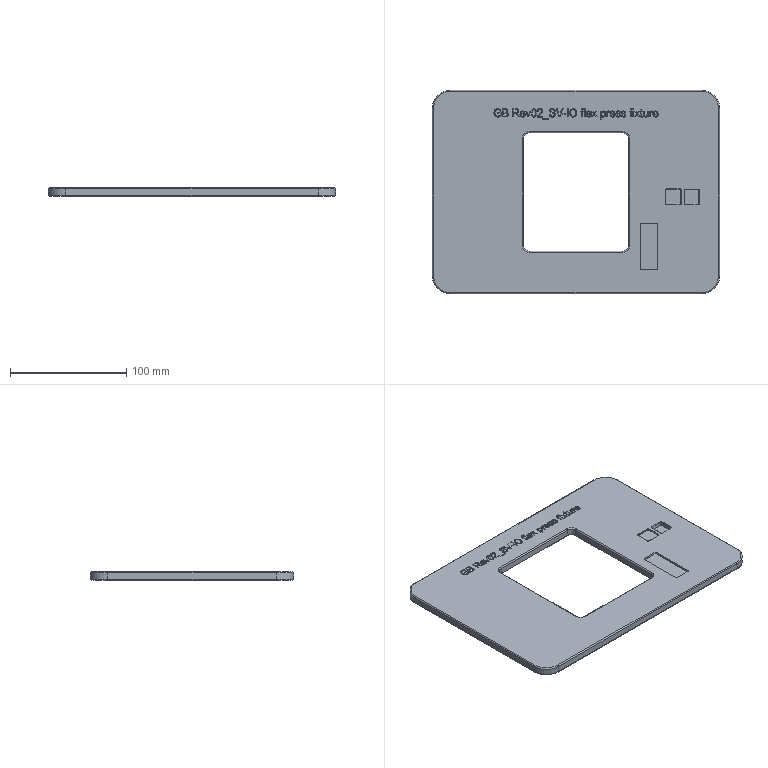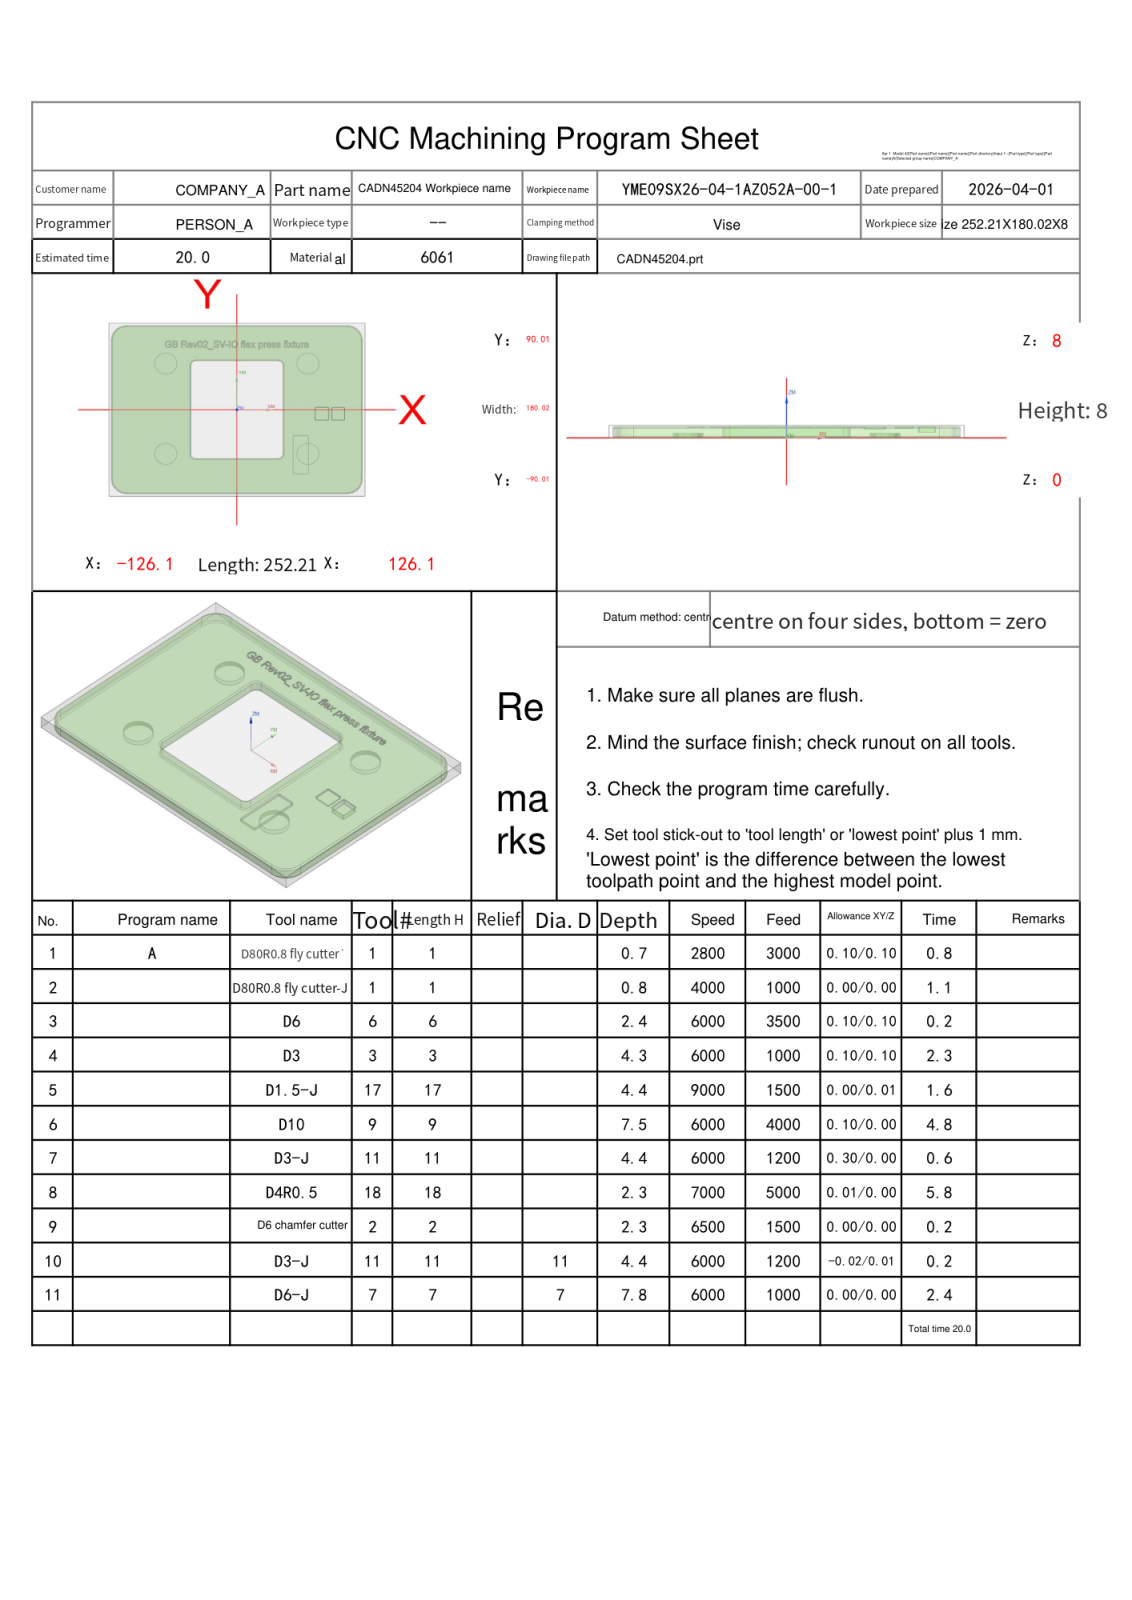NC program | NX | posted by the shop | part box 247.208 x 175.016 x 7.2 mm
Lines 7607 to 9197 of 29502:
N8 T18 M06
(D4R0.5  D=4. R=0.5 H=18 ce=0.01 di=0.00)
G00 G90 G54 X-18.349 Y50.167 M03 S7000
G43 H18 Z27.2
M08
Z8.7
G01 X-40.567 Z7.536 F5000.
X-41.143 Y50.101 Z7.505
X-41.705 Y49.958 Z7.475
X-42.242 Y49.741 Z7.444
X-42.746 Y49.455 Z7.414
X-43.207 Y49.103 Z7.384
X-43.617 Y48.693 Z7.353
X-43.968 Y48.232 Z7.323
X-44.255 Y47.729 Z7.293
X-44.472 Y47.191 Z7.262
X-44.615 Y46.629 Z7.232
X-44.681 Y46.054 Z7.201
Y45.846 Z7.191
Y-45.846
G03 X-40.359 Y-50.167 I4.322 J0.0
G01 X40.363
G03 X44.685 Y-45.846 I0.0 J4.322
G01 Y45.846
G03 X40.363 Y50.167 I-4.322 J0.0
G01 X-40.359
G03 X-44.681 Y45.846 I0.0 J-4.322
G01 X-44.682 Y43.852 Z7.19
X-44.68 Y41.859
Y39.866
X-44.679 Y37.872
Y35.879
X-44.678 Y33.886
X-44.677 Y31.893
X-44.676 Y29.899
Y27.906
X-44.675 Y25.913
X-44.674 Y23.919
X-44.673 Y21.926
X-44.672 Y19.933 Z7.189
Y17.94
X-44.671 Y15.946
X-44.67 Y13.953
X-44.669 Y11.96
Y9.966
X-44.668 Y7.973
X-44.667 Y5.98
X-44.666 Y3.987
Y1.993
X-44.665 Y0.0
X-44.664 Y-1.993
Y-3.987 Z7.188
X-44.663 Y-5.98
Y-7.973
X-44.662 Y-9.966
X-44.661 Y-11.96
X-44.66 Y-13.953
Y-15.946
X-44.659 Y-17.94
Y-19.933
X-44.658 Y-21.926
Y-23.919
X-44.656 Y-25.913 Z7.187
Y-27.906
X-44.655 Y-29.899
Y-31.893
X-44.654 Y-33.886
Y-35.879
X-44.653 Y-37.872
Y-39.866
X-44.651 Y-41.859
Y-43.852
X-44.65 Y-45.846
X-44.645 Y-46.044
X-44.632 Y-46.241
X-44.609 Y-46.438
X-44.577 Y-46.634
X-44.536 Y-46.828
X-44.486 Y-47.02
X-44.427 Y-47.209
X-44.36 Y-47.395
X-44.284 Y-47.578
X-44.2 Y-47.758
X-44.107 Y-47.933
X-44.007 Y-48.104
X-43.898 Y-48.27
X-43.783 Y-48.431
X-43.659 Y-48.586
X-43.53 Y-48.736
X-43.392 Y-48.879 Z7.186
X-43.249 Y-49.016
X-43.1 Y-49.145
X-42.944 Y-49.269
X-42.783 Y-49.384
X-42.618 Y-49.492
X-42.446 Y-49.593
X-42.271 Y-49.685
X-42.092 Y-49.769
X-41.909 Y-49.845
X-41.722 Y-49.912
X-41.533 Y-49.971
X-41.341 Y-50.02
X-41.148 Y-50.061
X-40.952 Y-50.093
X-40.755 Y-50.116
X-40.557 Y-50.129
X-40.359 Y-50.134
X-38.437
X-36.515 Y-50.133
X-34.594
X-32.672 Y-50.132
X-30.75
X-28.828 Y-50.131
X-26.906
X-24.984 Y-50.129
X-23.062 Y-50.13
X-21.14 Y-50.128
X-19.218 Z7.185
X-17.296 Y-50.127
X-15.374
X-13.452 Y-50.126
X-11.53
X-9.608 Y-50.125
X-7.686
X-5.764 Y-50.124
X-3.842
X-1.92 Y-50.122
X.002 Y-50.123
X1.924 Y-50.121
X3.846 Z7.184
X5.768 Y-50.12
X7.69
X9.612 Y-50.119
X11.534
X13.456 Y-50.118
X15.378
X17.3 Y-50.116
X19.222 Y-50.117
X21.144 Y-50.115
X23.066
X24.987 Y-50.114
X26.909 Z7.183
X28.831 Y-50.113
X30.753
X32.675 Y-50.112
X34.597
X36.519 Y-50.111
X38.441
X40.363 Y-50.11
X40.56 Y-50.105
X40.757 Y-50.092
X40.952 Y-50.069
X41.147 Y-50.037
X41.339 Y-49.996
X41.53 Y-49.947
X41.718 Y-49.889
X41.904 Y-49.822
X42.085 Y-49.746
X42.264 Y-49.662
X42.438 Y-49.57
X42.608 Y-49.471
X42.773 Y-49.363
X42.933 Y-49.248
X43.087 Y-49.126
X43.236 Y-48.996
X43.378 Y-48.86
X43.514 Y-48.718
X43.643 Y-48.569
X43.765 Y-48.415
X43.88 Y-48.255
X43.988 Y-48.09
X44.088 Y-47.92
X44.179 Y-47.746
X44.263 Y-47.567
X44.338 Y-47.386
X44.405 Y-47.2
X44.463 Y-47.012
X44.513 Y-46.822
X44.553 Y-46.629
X44.585 Y-46.434
X44.608 Y-46.239
X44.621 Y-46.042
X44.626 Y-45.846
X44.625 Y-43.852
Y-41.859 Z7.182
X44.624 Y-39.866
Y-37.872
X44.623 Y-35.879
Y-33.886
X44.622 Y-31.893
Y-29.899
X44.621 Y-27.906
Y-25.913
X44.62 Y-23.919
X44.619 Y-21.926
Y-19.933
X44.618 Y-17.94 Z7.181
Y-15.946
X44.617 Y-13.953
Y-11.96
X44.616 Y-9.966
Y-7.973
X44.615 Y-5.98
Y-3.987
X44.614 Y-1.993
Y0.0
X44.613 Y1.993
Y3.987 Z7.18
X44.612 Y5.98
Y7.973
X44.611 Y9.966
Y11.96
X44.61 Y13.953
Y15.946
X44.609 Y17.94
Y19.933
X44.608 Y21.926
Y23.919
X44.607 Y25.913
Y27.906 Z7.179
X44.606 Y29.899
Y31.893
X44.605 Y33.886
Y35.879
X44.604 Y37.872
Y39.866
X44.602 Y41.859
X44.603 Y43.852
X44.601 Y45.846
X44.597 Y46.041
X44.583 Y46.237
X44.561 Y46.431
X44.529 Y46.624
X44.489 Y46.816
X44.439 Y47.005
X44.381 Y47.192
X44.315 Y47.376
X44.24 Y47.557
X44.157 Y47.734
X44.065 Y47.908
X43.966 Y48.076
X43.859 Y48.24
X43.745 Y48.399
X43.623 Y48.553
X43.495 Y48.7
X43.36 Y48.842
X43.218 Y48.977
X43.07 Y49.106
X42.917 Y49.227
X42.758 Y49.341
X42.594 Y49.448
X42.425 Y49.547
X42.252 Y49.638 Z7.178
X42.075 Y49.722
X41.894 Y49.796
X41.71 Y49.863
X41.523 Y49.921
X41.333 Y49.97
X41.142 Y50.01
X40.949 Y50.042
X40.754 Y50.064
X40.559 Y50.078
X40.363 Y50.082
X38.441 Y50.083
X36.519 Y50.081
X34.597 Y50.082
X32.675 Y50.08
X30.753 Y50.081
X28.831 Y50.079
X26.909 Y50.08
X24.987 Y50.078
X23.066 Y50.079
X21.144 Y50.078
X19.222
X17.3 Y50.077 Z7.177
X15.378
X13.456 Y50.076
X11.534
X9.612 Y50.075
X7.69
X5.768 Y50.074
X3.846
X1.924 Y50.073
X.002
X-1.92 Y50.072
X-3.842
X-5.764 Y50.071 Z7.176
X-7.686
X-9.608 Y50.07
X-11.53
X-13.452 Y50.069
X-15.374
X-17.296
X-19.218 Y50.068
X-21.14
X-23.062 Y50.067
X-24.984
X-26.906 Y50.066
X-28.828 Z7.175
X-30.75 Y50.065
X-32.672
X-34.594 Y50.064
X-36.515
X-38.437
X-40.359 Y50.063
X-40.554 Y50.058
X-40.749 Y50.045
X-40.942 Y50.022
X-41.134 Y49.991
X-41.325 Y49.951
X-41.514 Y49.902
X-41.7 Y49.844
X-41.883 Y49.778
X-42.063 Y49.703
X-42.239 Y49.621
X-42.411 Y49.529
X-42.579 Y49.431
X-42.742 Y49.324
X-42.901 Y49.211
X-43.053 Y49.09
X-43.2 Y48.962
X-43.341 Y48.827
X-43.476 Y48.686
X-43.603 Y48.539
X-43.724 Y48.387
X-43.838 Y48.228
X-43.944 Y48.065
X-44.043 Y47.897
X-44.134 Y47.725
X-44.216 Y47.549
X-44.291 Y47.369
X-44.357 Y47.185
X-44.415 Y46.999
X-44.463 Y46.811
X-44.504 Y46.62
X-44.535 Y46.428
X-44.558 Y46.235
X-44.571 Y46.04
X-44.575 Y45.846
Y43.852
X-44.574 Y41.859 Z7.174
X-44.573 Y39.866
Y37.872
X-44.572 Y35.879
Y33.886
X-44.571 Y31.893
X-44.57 Y29.899
X-44.569 Y27.906
Y25.913 Z7.173
X-44.568 Y23.919
Y21.926
X-44.567 Y19.933
X-44.566 Y17.94
Y15.946
X-44.565 Y13.953
Y11.96
X-44.564 Y9.966
Y7.973 Z7.172
X-44.563 Y5.98
X-44.562 Y3.987
X-44.561 Y1.993
Y0.0
X-44.56 Y-1.993
Y-3.987
X-44.559 Y-5.98
Y-7.973 Z7.171
X-44.558 Y-9.966
Y-11.96
X-44.556 Y-13.953
X-44.557 Y-15.946
X-44.555 Y-17.94
Y-19.933
X-44.554 Y-21.926
Y-23.919 Z7.17
X-44.553 Y-25.913
Y-27.906
X-44.552 Y-29.899
Y-31.893
X-44.55 Y-33.886
X-44.551 Y-35.879
X-44.549 Y-37.872
Y-39.866 Z7.169
X-44.548 Y-41.859
Y-43.852
X-44.547 Y-45.846
X-44.542 Y-46.039
X-44.529 Y-46.232
X-44.507 Y-46.424
X-44.476 Y-46.615
X-44.435 Y-46.804
X-44.387 Y-46.991
X-44.329 Y-47.176
X-44.264 Y-47.358
X-44.19 Y-47.537
X-44.108 Y-47.712
X-44.017 Y-47.883
X-43.919 Y-48.05
X-43.813 Y-48.212
X-43.701 Y-48.369
X-43.58 Y-48.52
X-43.453 Y-48.666
X-43.32 Y-48.806
X-43.18 Y-48.94
X-43.034 Y-49.066
X-42.882 Y-49.186
X-42.725 Y-49.299
X-42.563 Y-49.405
X-42.396 Y-49.503
X-42.225 Y-49.593
X-42.05 Y-49.675
X-41.872 Y-49.749
X-41.69 Y-49.814
X-41.505 Y-49.872
X-41.318 Y-49.92
X-41.129 Y-49.96
X-40.938 Y-49.991
X-40.746 Y-50.014
X-40.553 Y-50.027
X-40.359 Y-50.031
X-38.437
X-36.515 Y-50.03
X-34.594 Z7.168
X-32.672 Y-50.029
X-30.75
X-28.828 Y-50.028
X-26.906
X-24.984 Y-50.027
X-23.062
X-21.14 Y-50.026
X-19.218 Z7.167
X-17.296 Y-50.025
X-15.374 Y-50.024
X-13.452
X-11.53 Y-50.023
X-9.608 Y-50.022
X-7.686
X-5.764 Y-50.021
X-3.842
X-1.92 Y-50.02 Z7.166
X.002
X1.924 Y-50.019
X3.846
X5.768 Y-50.018
X7.69
X9.612 Y-50.017
X11.534
X13.456 Y-50.016 Z7.165
X15.378 Y-50.015
X17.3
X19.222 Y-50.014
X21.144
X23.066 Y-50.013
X24.987
X26.909 Y-50.012
X28.831 Y-50.011
X30.753 Z7.164
X32.675 Y-50.01
X34.597
X36.519 Y-50.009
X38.441
X40.363 Y-50.008
X40.555 Y-50.004
X40.747 Y-49.991
X40.938 Y-49.969
X41.128 Y-49.937
X41.316 Y-49.898
X41.502 Y-49.849
X41.686 Y-49.792
X41.867 Y-49.727
X42.045 Y-49.653
X42.219 Y-49.571
X42.389 Y-49.482
X42.554 Y-49.384
X42.716 Y-49.279
X42.871 Y-49.167
X43.022 Y-49.048
X43.167 Y-48.921
X43.306 Y-48.789
X43.439 Y-48.649
X43.565 Y-48.504
X43.684 Y-48.354
X43.797 Y-48.198
X43.902 Y-48.036
X43.999 Y-47.871
X44.089 Y-47.701
X44.17 Y-47.527
X44.244 Y-47.349
X44.309 Y-47.168
X44.366 Y-46.984
X44.414 Y-46.798
X44.454 Y-46.61
X44.485 Y-46.42 Z7.163
X44.507 Y-46.23
X44.52 Y-46.038
X44.524 Y-45.846
Y-43.852
X44.523 Y-41.859
Y-39.866
X44.522 Y-37.872
Y-35.879
X44.521 Y-33.886
Y-31.893
X44.52 Y-29.899 Z7.162
Y-27.906
X44.519 Y-25.913
Y-23.919
X44.518 Y-21.926
Y-19.933
X44.517 Y-17.94
Y-15.946
X44.516 Y-13.953
Y-11.96 Z7.161
X44.515 Y-9.966
Y-7.973
X44.514 Y-5.98
Y-3.987
X44.513 Y-1.993
Y0.0
X44.512 Y1.993
Y3.987 Z7.16
X44.511 Y5.98
Y7.973
X44.51 Y9.966
Y11.96
X44.509 Y13.953
Y15.946
X44.508 Y17.94
Y19.933 Z7.159
X44.507 Y21.926
Y23.919
X44.506 Y25.913
Y27.906
X44.505 Y29.899
Y31.893
X44.504 Y33.886
Y35.879
X44.503 Y37.872 Z7.158
Y39.866
X44.502 Y41.859
Y43.852
X44.501 Y45.846
X44.496 Y46.037
X44.483 Y46.227
X44.461 Y46.417
X44.43 Y46.606
X44.391 Y46.793
X44.342 Y46.978
X44.286 Y47.16
X44.221 Y47.34
X44.148 Y47.517
X44.066 Y47.689
X43.977 Y47.859
X43.88 Y48.023
X43.776 Y48.183
X43.664 Y48.338
X43.546 Y48.488
X43.42 Y48.632
X43.288 Y48.771
X43.15 Y48.902
X43.006 Y49.028
X42.856 Y49.146
X42.701 Y49.258
X42.541 Y49.362
X42.376 Y49.459
X42.207 Y49.548
X42.034 Y49.629
X41.857 Y49.702
X41.678 Y49.767
X41.495 Y49.824
X41.31 Y49.872
X41.123 Y49.911
X40.935 Y49.942
X40.745 Y49.964
X40.554 Y49.977
X40.363 Y49.981
X38.441 Z7.157
X36.519 Y49.98
X34.597
X32.675 Y49.979
X30.753
X28.831 Y49.978
X26.909
X24.987 Y49.977
X23.066 Z7.156
X21.144 Y49.976
X19.222
X17.3
X15.378
X13.456 Y49.975
X11.534
X9.612 Y49.974
X7.69
X5.768 Y49.973 Z7.155
X3.846
X1.924 Y49.972
X.002
X-1.92 Y49.971
X-3.842
X-5.764 Y49.97
X-7.686
X-9.608 Y49.969 Z7.154
X-11.53
X-13.452 Y49.968
X-15.374
X-17.296 Y49.967
X-19.218
X-21.14 Y49.966
X-23.062
X-24.984
X-26.906 Y49.965 Z7.153
X-28.828
X-30.75 Y49.964
X-32.672
X-34.594 Y49.963
X-36.515
X-38.437 Y49.962
X-40.359
X-40.55 Y49.957
X-40.739 Y49.944
X-40.928 Y49.922
X-41.116 Y49.892
X-41.302 Y49.852
X-41.486 Y49.805
X-41.667 Y49.748
X-41.846 Y49.684
X-42.022 Y49.611
X-42.194 Y49.53
X-42.362 Y49.441
X-42.526 Y49.345 Z7.152
X-42.685 Y49.241
X-42.84 Y49.13
X-42.989 Y49.012
X-43.132 Y48.887
X-43.27 Y48.756
X-43.401 Y48.618
X-43.526 Y48.475
X-43.644 Y48.326
X-43.755 Y48.171
X-43.858 Y48.012
X-43.955 Y47.848
X-44.043 Y47.68
X-44.124 Y47.508
X-44.197 Y47.332
X-44.261 Y47.153
X-44.317 Y46.972
X-44.365 Y46.788
X-44.404 Y46.602
X-44.435 Y46.414
X-44.457 Y46.225
X-44.47 Y46.036
X-44.474 Y45.846
Y43.852
X-44.473 Y41.859
X-44.472 Y39.866
Y37.872
X-44.471 Y35.879 Z7.151
Y33.886
X-44.47 Y31.893
X-44.469 Y29.899
Y27.906
X-44.468 Y25.913
Y23.919
X-44.467 Y21.926 Z7.15
Y19.933
X-44.466 Y17.94
Y15.946
X-44.465 Y13.953
Y11.96
X-44.464 Y9.966 Z7.149
X-44.463 Y7.973
X-44.462 Y5.98
Y3.987
X-44.461 Y1.993
Y0.0
X-44.46 Y-1.993
Y-3.987 Z7.148
X-44.459 Y-5.98
Y-7.973
X-44.458 Y-9.966
Y-11.96
X-44.456 Y-13.953
X-44.457 Y-15.946 Z7.147
X-44.455 Y-17.94
Y-19.933
X-44.454 Y-21.926
Y-23.919
X-44.453 Y-25.913
Y-27.906 Z7.146
X-44.452 Y-29.899
Y-31.893
X-44.451 Y-33.886
Y-35.879
X-44.45 Y-37.872
Y-39.866
X-44.449 Y-41.859 Z7.145
Y-43.852
X-44.448 Y-45.846
X-44.442 Y-46.046
X-44.428 Y-46.246
X-44.403 Y-46.445
X-44.369 Y-46.643
X-44.325 Y-46.839
X-44.271 Y-47.032
X-44.208 Y-47.223
X-44.136 Y-47.41
X-44.054 Y-47.593
X-43.964 Y-47.772
X-43.865 Y-47.947
X-43.758 Y-48.116
X-43.642 Y-48.28
X-43.519 Y-48.439
X-43.388 Y-48.59
X-43.25 Y-48.736
X-43.104 Y-48.874
X-42.952 Y-49.005
X-42.794 Y-49.128
X-42.63 Y-49.244
X-42.46 Y-49.351
X-42.286 Y-49.45
X-42.107 Y-49.54
X-41.923 Y-49.621
X-41.736 Y-49.693
X-41.546 Y-49.756
X-41.352 Y-49.81
X-41.157 Y-49.854
X-40.959 Y-49.888
X-40.76 Y-49.912
X-40.56 Y-49.927
X-40.359 Y-49.932
X-38.437 Z7.144
X-36.515 Y-49.931
X-34.594
X-32.672 Y-49.93
X-30.75
X-28.828 Y-49.929
X-26.906 Y-49.928
X-24.984 Z7.143
X-23.062 Y-49.927
X-21.14
X-19.218 Y-49.926
X-17.296
X-15.374 Y-49.925
X-13.452 Z7.142
X-11.53 Y-49.924
X-9.608 Y-49.923
X-7.686
X-5.764 Y-49.922
X-3.842
X-1.92 Y-49.921
X.002 Z7.141
X1.924 Y-49.92
X3.846
X5.768 Y-49.919
X7.69
X9.612 Y-49.918
X11.534 Y-49.917
X13.456 Z7.14
X15.378 Y-49.916
X17.3
X19.222
X21.144 Y-49.915
X23.066
X24.987 Y-49.914
X26.909 Z7.139
X28.831 Y-49.913
X30.753
X32.675 Y-49.912
X34.597
X36.519 Y-49.911
X38.441 Z7.138
X40.363 Y-49.91
X40.563 Y-49.905
X40.762 Y-49.89
X40.96 Y-49.866
X41.156 Y-49.832
X41.351 Y-49.788
X41.543 Y-49.735
X41.732 Y-49.672
X41.918 Y-49.6
X42.101 Y-49.519
X42.279 Y-49.429
X42.452 Y-49.331
X42.621 Y-49.224
X42.784 Y-49.11
X42.941 Y-48.987
X43.092 Y-48.856
X43.237 Y-48.719
X43.374 Y-48.574
X43.504 Y-48.423
X43.627 Y-48.266
X43.742 Y-48.103
X43.848 Y-47.934
X43.947 Y-47.761
X44.036 Y-47.583
X44.117 Y-47.4
X44.189 Y-47.214
X44.251 Y-47.025
X44.304 Y-46.833
X44.348 Y-46.638
X44.382 Y-46.442
X44.406 Y-46.244
X44.421 Y-46.045
X44.426 Y-45.846
Y-43.852
X44.425 Y-41.859 Z7.137
Y-39.866
X44.424 Y-37.872
Y-35.879
X44.423 Y-33.886
Y-31.893
X44.422 Y-29.899
Y-27.906 Z7.136
X44.421 Y-25.913
Y-23.919
X44.42 Y-21.926
Y-19.933
X44.419 Y-17.94
Y-15.946 Z7.135
X44.418 Y-13.953
Y-11.96
X44.417 Y-9.966
Y-7.973
X44.416 Y-5.98
Y-3.987
X44.415 Y-1.993 Z7.134
Y0.0
X44.414 Y1.993
Y3.987
X44.413 Y5.98
Y7.973
X44.412 Y9.966 Z7.133
Y11.96
X44.411 Y13.953
Y15.946
X44.41 Y17.94
Y19.933
X44.409 Y21.926
Y23.919 Z7.132
X44.408 Y25.913
Y27.906
X44.407 Y29.899
Y31.893
X44.406 Y33.886
Y35.879 Z7.131
X44.405 Y37.872
Y39.866
X44.404 Y41.859
Y43.852
X44.403 Y45.846
X44.398 Y46.044
X44.383 Y46.241
X44.359 Y46.438
X44.325 Y46.634
X44.281 Y46.827
X44.228 Y47.018
X44.166 Y47.206
X44.095 Y47.391
X44.014 Y47.572
X43.925 Y47.749
X43.827 Y47.922 Z7.13
X43.721 Y48.089
X43.607 Y48.251
X43.485 Y48.408
X43.356 Y48.558
X43.219 Y48.701
X43.075 Y48.838
X42.925 Y48.967
X42.769 Y49.089
X42.607 Y49.203
X42.439 Y49.309
X42.267 Y49.407
X42.09 Y49.496
X41.909 Y49.576
X41.724 Y49.648
X41.535 Y49.71
X41.344 Y49.763
X41.151 Y49.806
X40.956 Y49.84
X40.759 Y49.864
X40.561 Y49.879
X40.363 Y49.883
X38.441
X36.519 Y49.882
X34.597
X32.675 Y49.881
X30.753 Y49.882 Z7.129
X28.831 Y49.88
X26.909 Y49.881
X24.987 Y49.879
X23.066 Y49.88
X21.144 Y49.879
X19.222
X17.3 Y49.878 Z7.128
X15.378
X13.456 Y49.877
X11.534
X9.612 Y49.876
X7.69
X5.768 Y49.875 Z7.127
X3.846
X1.924 Y49.874
X.002
X-1.92 Y49.873
X-3.842
X-5.764 Y49.872
X-7.686 Z7.126
X-9.608 Y49.871
X-11.53
X-13.452 Y49.87
X-15.374
X-17.296
X-19.218 Y49.869
X-21.14 Z7.125
X-23.062 Y49.868
X-24.984
X-26.906 Y49.867
X-28.828
X-30.75
X-32.672 Y49.866 Z7.124
X-34.594
X-36.515 Y49.865
X-38.437
X-40.359 Y49.864
X-40.557 Y49.859
X-40.753 Y49.845
X-40.949 Y49.82
X-41.143 Y49.787
X-41.336 Y49.743
X-41.526 Y49.691
X-41.713 Y49.629
X-41.897 Y49.558
X-42.077 Y49.478
X-42.254 Y49.389
X-42.425 Y49.292
X-42.592 Y49.186
X-42.753 Y49.073
X-42.908 Y48.951
X-43.058 Y48.822
X-43.2 Y48.687
X-43.336 Y48.544
X-43.465 Y48.394
X-43.586 Y48.239
X-43.7 Y48.078
X-43.805 Y47.911
X-43.903 Y47.739
X-43.991 Y47.563
X-44.071 Y47.383
X-44.142 Y47.199 Z7.123
X-44.204 Y47.012
X-44.256 Y46.822
X-44.299 Y46.629
X-44.333 Y46.435
X-44.357 Y46.239
X-44.371 Y46.043
X-44.376 Y45.846
Y43.852
X-44.375 Y41.859
Y39.866
X-44.374 Y37.872
Y35.879 Z7.122
X-44.373 Y33.886
Y31.893
X-44.372 Y29.899
Y27.906
X-44.371 Y25.913 Z7.121
X-44.37 Y23.919
Y21.926
X-44.369 Y19.933
X-44.368 Y17.94
Y15.946
X-44.367 Y13.953 Z7.12
Y11.96
X-44.366 Y9.966
Y7.973
X-44.365 Y5.98
Y3.987 Z7.119
X-44.364 Y1.993
Y0.0
X-44.363 Y-1.993
Y-3.987
X-44.362 Y-5.98 Z7.118
Y-7.973
X-44.361 Y-9.966
Y-11.96
X-44.359 Y-13.953
Y-15.946
X-44.358 Y-17.94 Z7.117
Y-19.933
X-44.357 Y-21.926
Y-23.919
X-44.356 Y-25.913
Y-27.906 Z7.116
X-44.355 Y-29.899
Y-31.893
X-44.354 Y-33.886
Y-35.879
X-44.353 Y-37.872 Z7.115
Y-39.866
X-44.352 Y-41.859
Y-43.852
X-44.351 Y-45.846
X-44.346 Y-46.041
X-44.332 Y-46.237
X-44.307 Y-46.431
X-44.274 Y-46.624
X-44.231 Y-46.815
X-44.179 Y-47.004
X-44.117 Y-47.19
X-44.047 Y-47.373
X-43.967 Y-47.552 Z7.114
X-43.879 Y-47.727
X-43.782 Y-47.897
X-43.678 Y-48.063
X-43.565 Y-48.223
X-43.444 Y-48.377
X-43.316 Y-48.525
X-43.181 Y-48.667
X-43.039 Y-48.802
X-42.891 Y-48.93
X-42.736 Y-49.051
X-42.576 Y-49.163
X-42.411 Y-49.268
X-42.24 Y-49.365
X-42.065 Y-49.453
X-41.886 Y-49.532
X-41.704 Y-49.602
X-41.518 Y-49.664
X-41.329 Y-49.716
X-41.138 Y-49.759
X-40.945 Y-49.792
X-40.751 Y-49.816
X-40.555 Y-49.83
X-40.359 Y-49.835
X-38.437
X-36.515 Y-49.834
X-34.594
X-32.672 Y-49.833 Z7.113
X-30.75
X-28.828 Y-49.832
X-26.906
X-24.984 Y-49.831
X-23.062 Z7.112
X-21.14 Y-49.83
X-19.218
X-17.296 Y-49.829
X-15.374
X-13.452 Y-49.828
X-11.53 Z7.111
X-9.608 Y-49.827
X-7.686
X-5.764 Y-49.826
X-3.842
X-1.92 Y-49.825 Z7.11
X.002
X1.924 Y-49.824
X3.846
X5.768 Y-49.823
X7.69 Z7.109
X9.612 Y-49.822
X11.534
X13.456 Y-49.821
X15.378
X17.3 Y-49.82
X19.222 Z7.108
X21.144 Y-49.819
X23.066
X24.987 Y-49.818
X26.909
X28.831 Y-49.817 Z7.107
X30.753
X32.675 Y-49.816
X34.597
X36.519 Y-49.815
X38.441
X40.363 Y-49.814 Z7.106
X40.558 Y-49.809
X40.752 Y-49.795
X40.945 Y-49.771
X41.137 Y-49.738
X41.327 Y-49.695
X41.515 Y-49.643
X41.7 Y-49.582
X41.882 Y-49.512
X42.06 Y-49.433
X42.234 Y-49.345
X42.403 Y-49.249
X42.568 Y-49.145
X42.727 Y-49.033
X42.88 Y-48.913
X43.028 Y-48.785
X43.169 Y-48.651
X43.303 Y-48.51
X43.43 Y-48.363
X43.55 Y-48.209
X43.662 Y-48.05
X43.766 Y-47.885
X43.862 Y-47.716
X43.95 Y-47.542
X44.028 Y-47.364
X44.099 Y-47.182
X44.16 Y-46.997
X44.211 Y-46.81
X44.254 Y-46.619
X44.287 Y-46.428
X44.311 Y-46.234
X44.325 Y-46.04
X44.33 Y-45.846
Y-43.852
X44.329 Y-41.859 Z7.105
Y-39.866
X44.328 Y-37.872
Y-35.879
X44.327 Y-33.886
Y-31.893 Z7.104
X44.326 Y-29.899
Y-27.906
X44.325 Y-25.913
Y-23.919
X44.324 Y-21.926
Y-19.933 Z7.103
X44.323 Y-17.94
Y-15.946
X44.322 Y-13.953
Y-11.96
X44.321 Y-9.966 Z7.102
Y-7.973
X44.32 Y-5.98
Y-3.987
X44.319 Y-1.993
Y0.0 Z7.101
X44.318 Y1.993
Y3.987
X44.317 Y5.98
Y7.973
X44.316 Y9.966 Z7.1
Y11.96
X44.315 Y13.953
Y15.946
X44.314 Y17.94
Y19.933
X44.313 Y21.926 Z7.099
Y23.919
X44.312 Y25.913
Y27.906
X44.311 Y29.899
Y31.893 Z7.098
X44.31 Y33.886
Y35.879
X44.309 Y37.872
Y39.866
X44.308 Y41.859 Z7.097
Y43.852
X44.307 Y45.846
X44.302 Y46.039
X44.288 Y46.232
X44.264 Y46.424
X44.231 Y46.615
X44.189 Y46.804
X44.137 Y46.99
X44.076 Y47.174
X44.007 Y47.355
X43.928 Y47.532
X43.841 Y47.705
X43.746 Y47.873
X43.642 Y48.036
X43.531 Y48.195
X43.412 Y48.347
X43.285 Y48.494
X43.152 Y48.634
X43.011 Y48.767
X42.865 Y48.894
X42.712 Y49.013
X42.554 Y49.124
X42.39 Y49.228
X42.222 Y49.323
X42.049 Y49.41
X41.872 Y49.488
X41.692 Y49.558
X41.508 Y49.619
X41.321 Y49.67
X41.132 Y49.713
X40.942 Y49.746
X40.75 Y49.769
X40.557 Y49.783 Z7.096
X40.363 Y49.788
X38.441
X36.519 Y49.787
X34.597
X32.675 Y49.786
X30.753
X28.831 Y49.785 Z7.095
X26.909
X24.987 Y49.784
X23.066
X21.144 Y49.783
X19.222 Z7.094
X17.3 Y49.782
X15.378
X13.456
X11.534 Y49.781
X9.612
X7.69 Y49.78 Z7.093
X5.768
X3.846 Y49.779
X1.924
X.002 Y49.778
X-1.92 Z7.092
X-3.842 Y49.777
X-5.764
X-7.686
X-9.608 Y49.776
X-11.53
X-13.452 Y49.775 Z7.091
X-15.374
X-17.296 Y49.774
X-19.218
X-21.14
X-23.062 Y49.773 Z7.09
X-24.984
X-26.906 Y49.772
X-28.828
X-30.75 Y49.771
X-32.672
X-34.594 Y49.77 Z7.089
X-36.515
X-38.437 Y49.769
X-40.359
X-40.552 Y49.764
X-40.744 Y49.75
X-40.935 Y49.726
X-41.125 Y49.693
X-41.313 Y49.651
X-41.498 Y49.6
X-41.681 Y49.539
X-41.861 Y49.47
X-42.037 Y49.392
X-42.209 Y49.305
X-42.376 Y49.21
X-42.539 Y49.107
X-42.696 Y48.996
X-42.848 Y48.878
X-42.994 Y48.752
X-43.133 Y48.619
X-43.266 Y48.48 Z7.088
X-43.392 Y48.334
X-43.51 Y48.182
X-43.621 Y48.025
X-43.724 Y47.862
X-43.819 Y47.695
X-43.905 Y47.523
X-43.983 Y47.347
X-44.052 Y47.167
X-44.113 Y46.984
X-44.164 Y46.799
X-44.206 Y46.611
X-44.239 Y46.421
X-44.263 Y46.23
X-44.277 Y46.038
X-44.281 Y45.846
Y43.852
X-44.28 Y41.859
Y39.866
X-44.279 Y37.872 Z7.087
Y35.879
X-44.278 Y33.886
Y31.893
X-44.277 Y29.899 Z7.086
Y27.906
X-44.276 Y25.913
Y23.919
X-44.275 Y21.926
Y19.933 Z7.085
X-44.274 Y17.94
X-44.273 Y15.946
Y13.953
X-44.272 Y11.96 Z7.084
Y9.966
X-44.271 Y7.973
Y5.98
X-44.27 Y3.987
X-44.269 Y1.993 Z7.083
Y0.0
X-44.268 Y-1.993
Y-3.987
X-44.267 Y-5.98 Z7.082
Y-7.973
X-44.266 Y-9.966
Y-11.96
X-44.265 Y-13.953
Y-15.946 Z7.081
X-44.264 Y-17.94
Y-19.933
X-44.263 Y-21.926
Y-23.919 Z7.08
X-44.262 Y-25.913
X-44.261 Y-27.906
Y-29.899
X-44.26 Y-31.893
Y-33.886 Z7.079
X-44.259 Y-35.879
Y-37.872
X-44.258 Y-39.866
Y-41.859 Z7.078
X-44.257 Y-43.852
Y-45.846
X-44.252 Y-46.037
X-44.238 Y-46.228
X-44.215 Y-46.417
X-44.182 Y-46.606
X-44.14 Y-46.793
X-44.089 Y-46.977
X-44.029 Y-47.158
X-43.96 Y-47.337
X-43.882 Y-47.512
X-43.796 Y-47.683
X-43.702 Y-47.849
X-43.6 Y-48.011
X-43.489 Y-48.167
X-43.372 Y-48.318
X-43.247 Y-48.462
X-43.115 Y-48.601
X-42.976 Y-48.733
X-42.831 Y-48.858
X-42.681 Y-48.975
X-42.524 Y-49.085
X-42.363 Y-49.188 Z7.077
X-42.196 Y-49.282
X-42.025 Y-49.368
X-41.85 Y-49.445
X-41.672 Y-49.514
X-41.49 Y-49.574
X-41.306 Y-49.625
X-41.12 Y-49.667
X-40.931 Y-49.699
X-40.741 Y-49.723
X-40.551 Y-49.737
X-40.359 Y-49.742
X-38.437 Y-49.741
X-36.515
X-34.594 Y-49.74
X-32.672 Z7.076
X-30.75 Y-49.739
X-28.828
X-26.906 Y-49.738
X-24.984
X-23.062 Y-49.737 Z7.075
X-21.14
X-19.218 Y-49.736
X-17.296
X-15.374 Y-49.735 Z7.074
X-13.452
X-11.53 Y-49.734
X-9.608
X-7.686 Y-49.733
X-5.764 Z7.073
X-3.842 Y-49.732
X-1.92
X.002 Y-49.731
X1.924
X3.846 Y-49.73 Z7.072
X5.768
X7.69 Y-49.729
X9.612
X11.534 Y-49.728 Z7.071
X13.456
X15.378 Y-49.727
X17.3
X19.222 Y-49.726
X21.144 Z7.07
X23.066 Y-49.725
X24.987
X26.909 Y-49.724
X28.831
X30.753 Y-49.723 Z7.069
X32.675
X34.597 Y-49.722
X36.519
X38.441 Y-49.721 Z7.068
X40.363
X40.553 Y-49.716
X40.743 Y-49.702
X40.932 Y-49.679
X41.119 Y-49.646
X41.305 Y-49.605
X41.488 Y-49.554
X41.669 Y-49.494
X41.846 Y-49.425
X42.02 Y-49.349
X42.19 Y-49.263
X42.355 Y-49.169
X42.516 Y-49.067
X42.671 Y-48.958
X42.821 Y-48.841
X42.965 Y-48.717
X43.103 Y-48.585
X43.234 Y-48.448
X43.358 Y-48.303
X43.475 Y-48.154
X43.585 Y-47.998
X43.686 Y-47.837
X43.78 Y-47.672
X43.866 Y-47.502
X43.942 Y-47.328
X44.011 Y-47.151
X44.07 Y-46.97
X44.121 Y-46.787
X44.163 Y-46.601
X44.195 Y-46.414
X44.218 Y-46.225
X44.232 Y-46.036
X44.237 Y-45.846
Y-43.852 Z7.067
X44.236 Y-41.859
Y-39.866
X44.235 Y-37.872
Y-35.879 Z7.066
X44.234 Y-33.886
Y-31.893
X44.233 Y-29.899
Y-27.906
X44.232 Y-25.913 Z7.065
Y-23.919
X44.231 Y-21.926
Y-19.933
X44.23 Y-17.94 Z7.064
Y-15.946
X44.229 Y-13.953
Y-11.96
X44.228 Y-9.966
Y-7.973 Z7.063
X44.227 Y-5.98
Y-3.987
X44.226 Y-1.993
Y0.0 Z7.062
X44.225 Y1.993
Y3.987
X44.224 Y5.98
Y7.973
X44.223 Y9.966 Z7.061
Y11.96
X44.222 Y13.953
Y15.946
Y17.94 Z7.06
X44.221 Y19.933
Y21.926
X44.22 Y23.919
Y25.913
X44.219 Y27.906 Z7.059
Y29.899
X44.218 Y31.893
Y33.886
X44.217 Y35.879 Z7.058
Y37.872
X44.216 Y39.866
Y41.859
X44.215 Y43.852 Z7.057
Y45.846
X44.21 Y46.035
X44.196 Y46.223
X44.173 Y46.411
X44.141 Y46.597
X44.099 Y46.781
X44.049 Y46.964
X43.989 Y47.143
X43.921 Y47.319
X43.845 Y47.492
X43.76 Y47.661
X43.666 Y47.825
X43.565 Y47.985
X43.456 Y48.14
X43.34 Y48.289
X43.217 Y48.432
X43.086 Y48.569
X42.949 Y48.699
X42.806 Y48.822
X42.657 Y48.939
X42.503 Y49.047
X42.343 Y49.148
X42.178 Y49.241
X42.01 Y49.326
X41.837 Y49.403
X41.66 Y49.471
X41.481 Y49.53
X41.299 Y49.581
X41.114 Y49.622
X40.928 Y49.654
X40.741 Y49.677
X40.552 Y49.691
X40.363 Y49.696
X38.441 Y49.695 Z7.056
X36.519
X34.597
X32.675 Y49.694
X30.753
X28.831 Y49.693 Z7.055
X26.909
X24.987 Y49.692
X23.066
X21.144 Y49.691 Z7.054
X19.222
X17.3 Y49.69
X15.378
X13.456 Y49.689
X11.534 Z7.053
X9.612 Y49.688
X7.69
X5.768 Y49.687
X3.846
X1.924 Z7.052
X.002 Y49.686
X-1.92
X-3.842
X-5.764 Y49.685 Z7.051
X-7.686
X-9.608 Y49.684
X-11.53
X-13.452 Y49.683
X-15.374 Z7.05
X-17.296 Y49.682
X-19.218
X-21.14 Y49.681
X-23.062 Z7.049
X-24.984 Y49.68
X-26.906
X-28.828
X-30.75 Y49.679
X-32.672 Z7.048
X-34.594 Y49.678
X-36.515
X-38.437
X-40.359 Y49.677
X-40.547 Y49.672
X-40.735 Y49.658
X-40.922 Y49.635 Z7.047
X-41.107 Y49.603
X-41.29 Y49.562
X-41.472 Y49.512
X-41.65 Y49.453
X-41.825 Y49.385
X-41.997 Y49.309
X-42.165 Y49.224
X-42.329 Y49.131
X-42.488 Y49.031
X-42.641 Y48.922
X-42.79 Y48.807
X-42.932 Y48.684
X-43.068 Y48.554
X-43.198 Y48.418
X-43.321 Y48.276
X-43.436 Y48.127
X-43.544 Y47.974
X-43.645 Y47.815
X-43.738 Y47.651
X-43.822 Y47.483
X-43.898 Y47.311
X-43.966 Y47.136
X-44.025 Y46.957
X-44.075 Y46.776
X-44.116 Y46.593
X-44.148 Y46.408
X-44.171 Y46.221
X-44.185 Y46.034
X-44.189 Y45.846
Y43.852
X-44.188 Y41.859 Z7.046
Y39.866
X-44.187 Y37.872
Y35.879
X-44.186 Y33.886 Z7.045
Y31.893
X-44.185 Y29.899
Y27.906
X-44.184 Y25.913 Z7.044
Y23.919
X-44.183 Y21.926
Y19.933
X-44.182 Y17.94 Z7.043
Y15.946
X-44.181 Y13.953
Y11.96
X-44.18 Y9.966 Z7.042
Y7.973
X-44.179 Y5.98
Y3.987
X-44.178 Y1.993 Z7.041
Y0.0
X-44.177 Y-1.993
Y-3.987 Z7.04
X-44.176 Y-5.98
Y-7.973
X-44.175 Y-9.966